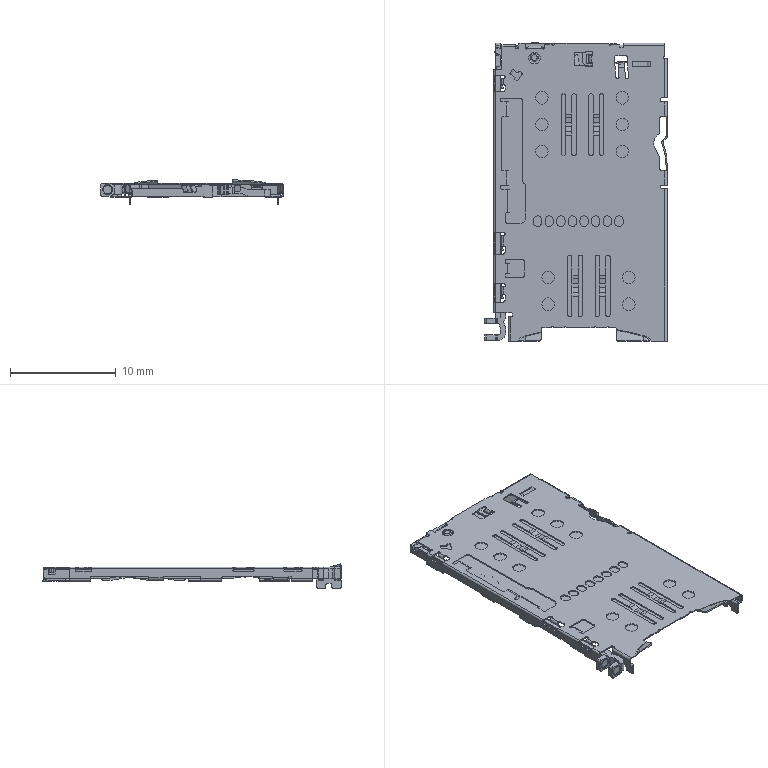Part | Creo | 1 solid | 1187 faces | box 17.275 x 28.25 x 2.305 mm | volume 74.352 mm3 | plane 593 | cylinder 534 | spline 30 | torus 18 | cone 8 | sphere 4 | commonest cylinder face diameters 0.3 x140 0.2 x132 1.2 x41 0.44 x30 0.1 x26 0.6 x16